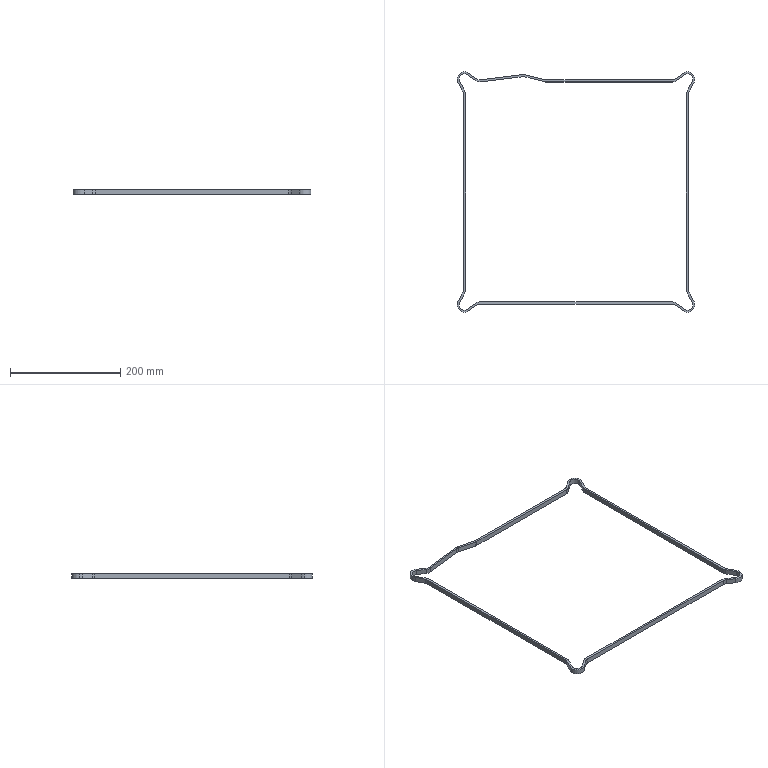Part | NX | features BREP 1 | 1 solid | 62 faces | box 431.47 x 436.47 x 9 mm | volume 59188 mm3 | cylinder 32 | plane 30 | commonest cylinder face diameters 19 x9 26.6 x9 18.87 x7 26.47 x7